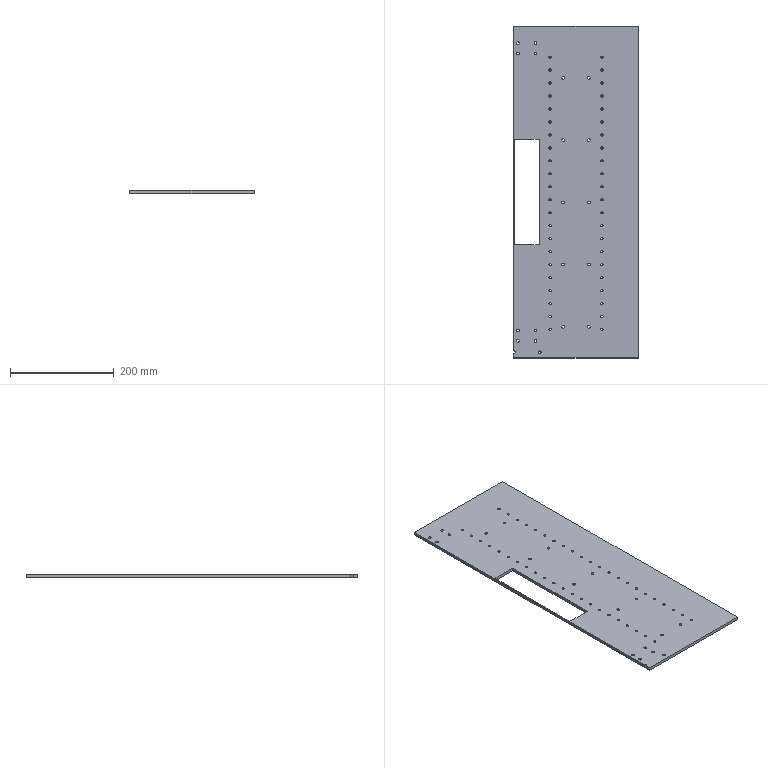Part | SolidWorks | features BaseBody 1 | 1 solid | 138 faces | box 240 x 640 x 6 mm | volume 856433 mm3 | cylinder 127 | plane 11 | commonest cylinder face diameters 4.3 x88 5.3 x39